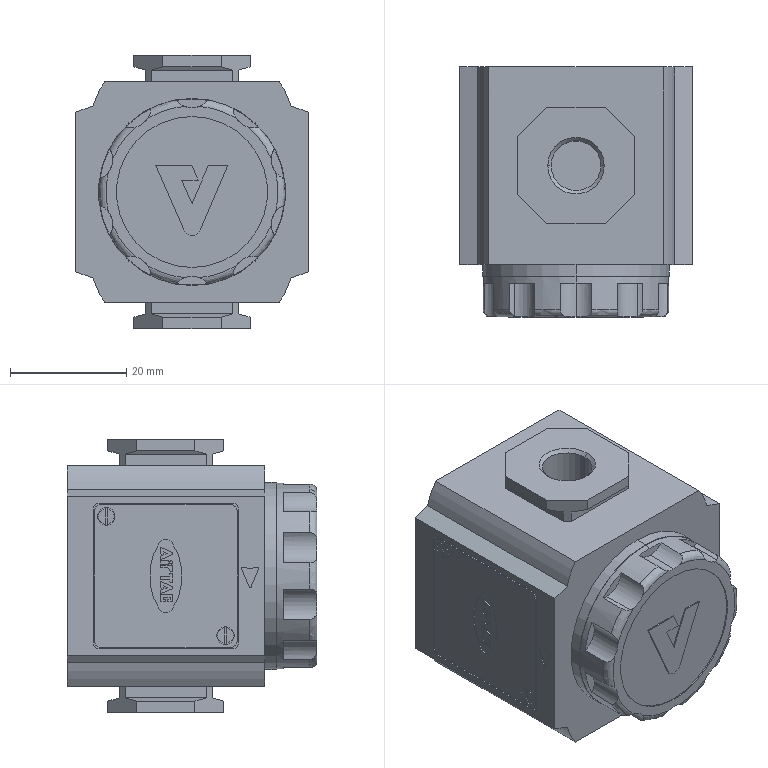Part | SolidWorks | features ICE 27, RefAxis 15, 3DProfileFeature 5, RevCut 2, Extrusion 1, LPattern 1, Revolution 1 | 1 solid | 267 faces | box 40 x 43 x 47 mm | volume 55436 mm3 | plane 157 | cylinder 96 | torus 10 | cone 4 | commonest cylinder face diameters 6.928 x13 2 x8 2.75 x8 3 x8 0.4 x6 0.488 x6